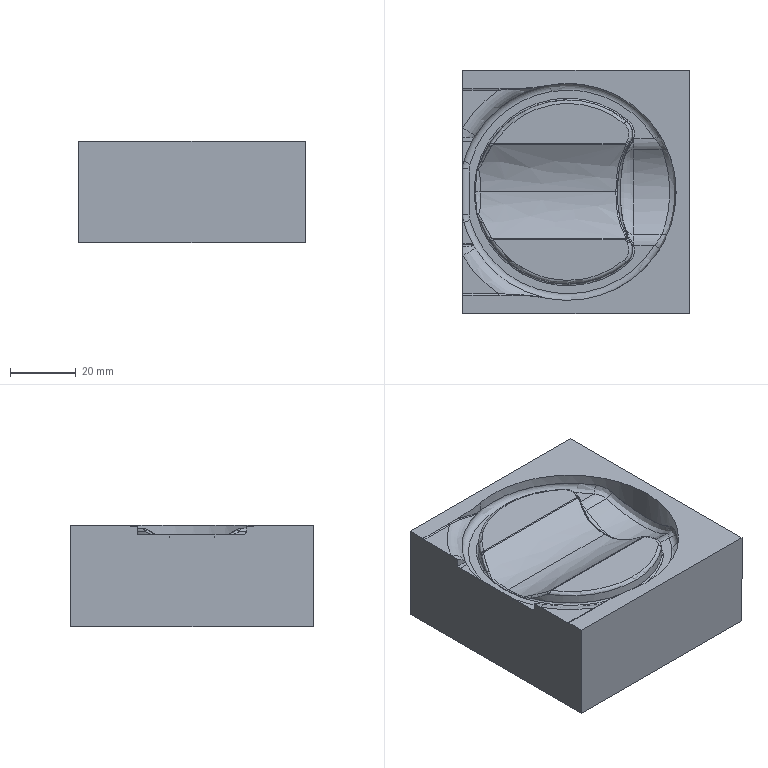NC program | NX | posted with a generic post | part box 69 x 74 x 31.001 mm
Lines 1 to 1116 of 31411:
N10 G17 G21 G94 G90
(CAVITY_MILL , TOOL : D10)
N12 T00 M6
N14 G54
N16 G17 G0 G90 X-5. Y37. S3000 M3
N18 G43 Z10.005 H0
N20 Z0.05
N22 G94 G1 Z-0.15 F2500.
N24 X26.
N26 Y36.067
N28 G2 X31.65 Y35.183 R81.15
N30 G3 X31.65 Y38.817 R-1.85
N32 G2 X26. Y37.933 R81.15
N34 G1 Y37.
N36 X19.5
N38 Y30.081
N40 G2 X30.42 Y28.801 R74.65
N42 G3 X30.42 Y45.199 R-8.35
N44 G2 X19.5 Y43.919 R74.65
N46 G1 Y37.
N48 X13.
N50 Y23.838
N52 G3 X15.404 Y23.65 R100.064
N54 G1 X16.292
N56 G2 X29.19 Y22.418 R68.15
N58 G3 X29.19 Y51.582 R-14.85
N60 G2 X16.292 Y50.35 R68.15
N62 G1 X15.325
N64 X13. Y50.167
N66 Y37.
N68 X6.5
N70 Y17.473
N72 X11.279
N74 X11.596 Y17.442
N76 G3 X15.193 Y17.15 R106.564
N78 G1 X16.292
N80 G2 X27.959 Y16.036 R61.65
N82 G3 X27.959 Y57.964 R-21.35
N84 G2 X16.292 Y56.85 R61.65
N86 G1 X15.069
N88 X10.976 Y56.527
N90 X6.5
N92 Y37.
N94 X0.
N96 Y10.973
N98 X10.961
N100 G3 X14.988 Y10.65 R113.064
N102 G1 X16.292
N104 G2 X26.729 Y9.653 R55.15
N106 G3 X26.729 Y64.347 R-27.85
N108 G2 X16.292 Y63.35 R55.15
N110 G1 X14.813
N112 X10.72 Y63.027
N114 X0.
N116 Y37.
N118 X-5.
N120 Z0.05
N122 G0 Z0.305
N124 Z-0.2
N126 G1 Z-0.4
N128 X33.85
N130 G3 X31.65 Y38.817 R1.85
N132 G2 X27.22 Y38.089 R81.15
N134 X26.569 Y37.006 R31.307
N136 X27.225 Y35.91 R31.167
N138 X31.65 Y35.183 R81.15
N140 G3 X33.85 Y37. R1.85
N142 G1 X40.35
N144 G3 X30.42 Y45.199 R8.35
N146 G2 X23.219 Y44.172 R74.65
N148 G3 X22.617 Y43.364 R11.338
N150 G1 X22.107 Y42.289
N152 G2 X19.5 Y38.251 R24.807
N154 G1 Y35.767
N156 G2 X22.41 Y31.101 R24.667
N158 G1 X22.67 Y30.558
N160 G3 X23.219 Y29.828 R11.338
N162 G2 X30.42 Y28.801 R74.65
N164 G3 X40.35 Y37. R8.35
N166 G1 X46.85
N168 G3 X29.19 Y51.582 R14.85
N170 G2 X20.304 Y50.468 R68.15
N172 G3 X16.935 Y46.55 R17.838
N174 G1 X16.288 Y45.188
N176 G2 X13. Y40.71 R18.307
N178 G1 Y33.31
N180 G2 X16.546 Y28.296 R18.167
N182 G1 X17.004 Y27.341
N184 G3 X20.304 Y23.532 R17.838
N186 G2 X29.19 Y22.418 R68.15
N188 G3 X46.85 Y37. R14.85
N190 G1 X53.35
N192 G3 X27.959 Y57.964 R21.35
N194 G2 X17.949 Y56.872 R61.65
N196 G3 X11.22 Y49.668 R24.338
N198 G1 X10.48 Y48.111
N200 G2 X6.5 Y43.763 R11.807
N202 G1 Y30.253
N204 G2 X10.682 Y25.492 R11.667
N206 G1 X11.303 Y24.195
N208 G3 X17.949 Y17.128 R24.338
N210 G2 X27.959 Y16.036 R61.65
N212 G3 X53.35 Y37. R21.35
N214 G1 X59.85
N216 G3 X26.729 Y64.347 R27.85
N218 G2 X16.292 Y63.35 R55.15
N220 G1 X16.095
N222 X15.926 Y63.318
N224 G3 X5.66 Y53.037 R30.838
N226 G1 X5.468 Y52.708
N228 X4.696 Y51.083
N230 G2 X0. Y48.349 R5.307
N232 G1 Y25.651
N234 G2 X0.837 Y25.584 R5.161
N236 X4.818 Y22.689 R5.167
N238 G1 X5.558 Y21.142
N240 X5.66 Y20.963
N242 G3 X15.979 Y10.65 R30.838
N244 G1 X16.292
N246 G2 X26.729 Y9.653 R55.15
N248 G3 X59.85 Y37. R27.85
N250 G1 X54.85
N252 Z-0.2
N254 G0 Z0.15
N256 X-5.
N258 Z-0.45
N260 G1 Z-0.65
N262 X33.85
N264 G3 X31.65 Y38.817 R1.85
N266 G2 X27.925 Y38.188 R81.15
N268 X27.213 Y36.999 R31.319
N270 X27.924 Y35.812 R31.317
N272 X31.65 Y35.183 R81.15
N274 G3 X33.85 Y37. R1.85
N276 G1 X40.35
N278 G3 X30.42 Y45.199 R8.35
N280 G2 X24.124 Y44.262 R74.65
N282 G3 X23.065 Y42.91 R10.713
N284 G2 X19.5 Y37.467 R24.819
N286 G1 Y36.532
N288 G2 X23.061 Y31.095 R24.817
N290 G3 X24.124 Y29.738 R10.713
N292 G2 X30.42 Y28.801 R74.65
N294 G3 X40.35 Y37. R8.35
N296 G1 X46.85
N298 G3 X29.19 Y51.582 R14.85
N300 G2 X21.372 Y50.54 R68.15
N302 G3 X17.359 Y46.052 R17.213
N304 G2 X13. Y40.094 R18.319
N306 G1 Y33.905
N308 G2 X17.355 Y27.955 R18.317
N310 G3 X21.372 Y23.46 R17.213
N312 G2 X29.19 Y22.418 R68.15
N314 G3 X46.85 Y37. R14.85
N316 G1 X53.35
N318 G3 X27.959 Y57.964 R21.35
N320 G2 X19.128 Y56.915 R61.65
N322 G3 X11.746 Y49.332 R23.713
N324 X11.483 Y48.832 R4.509
N326 G2 X6.5 Y43.371 R11.819
N328 G1 Y30.628
N330 G2 X11.477 Y25.178 R11.817
N332 G3 X11.746 Y24.668 R4.637
N334 X19.128 Y17.085 R23.713
N336 G2 X27.959 Y16.036 R61.65
N338 G3 X53.35 Y37. R21.35
N340 G1 X59.85
N342 G3 X26.729 Y64.347 R27.85
N344 G2 X17.233 Y63.358 R55.15
N346 G3 X6.194 Y52.712 R30.213
N348 X5.552 Y51.492 R11.009
N350 G2 X0.663 Y48.35 R5.319
N352 G1 X0.
N354 Y25.65
N356 X0.666
N358 G2 X5.549 Y22.513 R5.317
N360 G3 X6.194 Y21.288 R11.137
N362 X17.233 Y10.642 R30.213
N364 G2 X26.729 Y9.653 R55.15
N366 G3 X59.85 Y37. R27.85
N368 G1 X54.85
N370 Z-0.45
N372 G0 Z-0.1
N374 X-5.
N376 Z-0.7
N378 G1 Z-0.9
N380 X33.85
N382 G3 X31.65 Y38.817 R1.85
N384 G2 X28.439 Y38.264 R81.15
N386 X27.686 Y37. R31.284
N388 X28.438 Y35.736 R31.257
N390 X31.65 Y35.183 R81.15
N392 G3 X33.85 Y37. R1.85
N394 G1 X40.35
N396 G3 X30.42 Y45.199 R8.35
N398 G2 X24.823 Y44.339 R74.65
N400 G3 X23.424 Y42.641 R10.265
N402 G1 X22.973 Y41.811
N404 G2 X19.565 Y37.001 R24.784
N406 X22.955 Y32.22 R24.757
N408 G1 X23.421 Y31.364
N410 G3 X24.823 Y29.661 R10.265
N412 G2 X30.42 Y28.801 R74.65
N414 G3 X40.35 Y37. R8.35
N416 G1 X46.85
N418 G3 X29.19 Y51.582 R14.85
N420 G2 X22.206 Y50.607 R68.15
N422 G3 X17.826 Y45.954 R16.765
N424 G1 X17.261 Y44.912
N426 G2 X13. Y39.675 R18.284
N428 G1 Y34.329
N430 G2 X17.245 Y29.115 R18.257
N432 G1 X17.824 Y28.05
N434 G3 X22.206 Y23.393 R16.765
N436 G2 X29.19 Y22.418 R68.15
N438 G3 X46.85 Y37. R14.85
N440 G1 X53.35
N442 G3 X27.959 Y57.964 R21.35
N444 G2 X20.056 Y56.965 R61.65
N446 G3 X12.207 Y49.228 R23.265
N448 G1 X11.548 Y48.013
N450 G2 X6.5 Y43.114 R11.784
N452 G1 Y30.89
N454 G2 X11.534 Y26.01 R11.757
N456 G1 X12.206 Y24.774
N458 G3 X20.056 Y17.035 R23.265
N460 G2 X27.959 Y16.036 R61.65
N462 G3 X53.35 Y37. R21.35
N464 G1 X59.85
N466 G3 X26.729 Y64.347 R27.85
N468 G2 X18.221 Y63.384 R55.15
N470 G3 X6.576 Y52.479 R29.765
N472 G1 X5.835 Y51.113
N474 G2 X1.191 Y48.35 R5.284
N476 G1 X0.
N478 Y25.65
N480 X1.206
N482 G2 X5.824 Y22.904 R5.257
N484 G1 X6.576 Y21.521
N486 G3 X18.221 Y10.616 R29.765
N488 G2 X26.729 Y9.653 R55.15
N490 G3 X59.85 Y37. R27.85
N492 G1 X54.85
N494 Z-0.7
N496 G0 Z-0.35
N498 X-5. Y36.999
N500 Z-0.95
N502 G1 Z-1.15
N504 X6.5
N506 Y34.278
N508 G2 X8.893 Y34.52 R11.975
N510 G1 X49.414 Y34.521
N512 G2 X53.136 Y33.986 R12.122
N514 G3 X53.136 Y40.015 R21.35
N516 G2 X49.411 Y39.48 R12.106
N518 G1 X9.291
N520 X8.714 Y39.486
N522 G2 X6.5 Y39.719 R11.904
N524 G1 Y36.999
N526 X0.
N528 Y25.65
N530 X1.623
N532 G2 X4.035 Y25.069 R5.49
N534 X8.893 Y28.02 R5.475
N536 G1 X49.464 Y28.021
N538 G2 X54.095 Y25.737 R5.622
N540 G1 X54.555 Y25.01
N542 G2 X55.793 Y22.525 R11.904
N544 G3 X55.773 Y51.507 R27.85
N546 G2 X54.057 Y48.217 R12.539
N548 X49.464 Y45.98 R5.606
N550 G1 X9.327
N552 X8.786 Y45.986
N554 G2 X4.036 Y48.927 R5.404
N556 X1.617 Y48.35 R5.62
N558 G1 X0.
N560 Y36.999
N562 X-5.
N564 Z-0.95
N566 G0 Z-0.6
N568 Y37.001
N570 Z-1.2
N572 G1 Z-1.4
N574 X6.5
N576 Y34.758
N578 G2 X8.565 Y34.932 R11.933
N580 G1 X49.398 Y34.935
N582 G2 X53.184 Y34.344 R12.425
N584 G3 X53.184 Y39.655 R21.35
N586 G2 X49.401 Y39.065 R12.417
N588 G1 X8.561 Y39.068
N590 G2 X6.5 Y39.244 R11.951
N592 G1 Y37.001
N594 X0.
N596 Y25.65
N598 X1.979
N600 G2 X3.65 Y25.378 R5.705
N602 X8.555 Y28.432 R5.433
N604 G1 X49.399 Y28.435
N606 G2 X54.258 Y25.9 R5.925
N608 X55.949 Y22.784 R15.835
N610 G3 X55.952 Y51.21 R27.85
N612 G2 X54.285 Y48.139 R17.009
N614 X49.402 Y45.565 R5.917
N616 G1 X8.555 Y45.568
N618 G2 X3.649 Y48.619 R5.451
N620 X1.98 Y48.35 R6.113
N622 G1 X0.
N624 Y37.001
N626 X-5.
N628 Z-1.2
N630 G0 Z-0.85
N632 Y37. Z-1.45
N634 G1 Z-1.65
N636 X6.5
N638 Y35.216
N640 G2 X8.26 Y35.347 R11.898
N642 G1 X49.127
N644 G2 X53.222 Y34.666 R12.652
N646 G3 X53.222 Y39.335 R21.35
N648 G2 X49.116 Y38.653 R12.684
N650 G1 X8.259
N652 G2 X6.5 Y38.784 R11.896
N654 G1 Y37.
N656 X0.
N658 Y25.65
N660 X2.289
N662 X2.381 Y25.648
N664 X3.152 Y25.576
N666 X3.288 Y25.551
N668 G2 X8.26 Y28.847 R5.398
N670 G1 X49.127
N672 G2 X54.074 Y26.352 R6.152
N674 X56.034 Y22.928 R16.956
N676 G3 X56.027 Y51.083 R27.85
N678 G2 X54.111 Y47.69 R16.733
N680 X49.116 Y45.153 R6.184
N682 G1 X8.259
N684 G2 X3.289 Y48.448 R5.396
N686 X2.29 Y48.35 R5.432
N688 G1 X0.
N690 Y37.
N692 X-5.
N694 Z-1.45
N696 G0 Z-1.1
N698 Y37.001 Z-1.7
N700 G1 Z-1.9
N702 X6.5
N704 Y35.661
N706 G2 X8.034 Y35.759 R11.939
N708 G1 X48.917
N710 G2 X53.255 Y34.993 R12.654
N712 G3 X53.255 Y39.008 R21.35
N714 G2 X48.915 Y38.241 R12.654
N716 G1 X8.001 Y38.246
N718 G2 X6.5 Y38.341 R11.866
N720 G1 Y37.001
N722 X0.
N724 Y25.65
N726 X0.065
N728 X2.562
N730 X2.908 Y25.64
N732 G2 X8.034 Y29.259 R5.439
N734 G1 X48.917
N736 G2 X53.798 Y26.853 R6.154
N738 X56.067 Y22.986 R18.085
N740 G3 X56.066 Y51.015 R27.85
N742 G2 X53.81 Y47.162 R18.369
N744 X48.916 Y44.741 R6.154
N746 G1 X8.001 Y44.746
N748 G2 X2.932 Y48.353 R5.366
N750 G1 X2.562 Y48.35
N752 X0.
N754 Y37.001
N756 X-5.
N758 Z-1.7
N760 G0 Z-1.35
N762 Y36.999
N764 Z-1.95
N766 G1 Z-2.15
N768 X6.5
N770 Y36.099
N772 G2 X7.749 Y36.171 R11.965
N774 G1 X48.669 Y36.172
N776 G2 X53.284 Y35.323 R12.569
N778 G3 X53.284 Y38.676 R21.35
N780 G2 X48.668 Y37.828 R12.565
N782 G1 X7.781
N784 G2 X6.5 Y37.898 R11.903
N786 G1 Y36.999
N788 X0.
N790 Y25.706
N792 G2 X2.559 Y25.711 R40.064
N794 X7.784 Y29.672 R5.465
N796 G1 X48.692
N798 G2 X53.534 Y27.33 R6.069
N800 X56.082 Y23.011 R21.841
N802 G3 X56.078 Y50.996 R27.85
N804 G2 X53.534 Y46.67 R21.181
N806 X48.692 Y44.328 R6.065
N808 G1 X7.784
N810 G2 X2.564 Y48.35 R5.403
N812 G1 X0.
N814 Y36.999
N816 X-5.
N818 Z-1.95
N820 G0 Z-1.6
N822 Y37. Z-2.2
N824 G1 Z-2.4
N826 X6.5
N828 Y36.534
N830 G2 X7.591 Y36.583 R11.963
N832 G1 X48.779 Y36.582
N834 G2 X53.308 Y35.657 R12.355
N836 G3 X53.307 Y38.352 R21.35
N838 G2 X48.551 Y37.417 R12.557
N840 G1 X7.593 Y37.416
N842 G2 X6.5 Y37.466 R11.965
N844 G1 Y37.
N846 X0.
N848 Y25.824
N850 X0.065 Y25.823
N852 X1.978 Y25.826
N854 X2.261 Y25.82
N856 G2 X7.591 Y30.083 R5.463
N858 G1 X48.692
N860 G2 X52.593 Y28.523 R5.855
N862 X53.717 Y27.222 R7.773
N864 X56.092 Y23.028 R27.85
N866 G3 X56.088 Y50.979 R27.85
N868 G2 X53.46 Y46.426 R25.701
N870 X48.551 Y43.917 R6.057
N872 G1 X7.593 Y43.916
N874 G2 X2.226 Y48.35 R5.465
N876 G1 X0.
N878 Y37.
N880 X-5.
N882 Z-2.2
N884 G0 Z-1.85
N886 Z-2.45
N888 G1 Z-2.65
N890 X6.5
N892 Y36.966
N894 G2 X7.36 Y36.997 R11.955
N896 G1 X48.376 Y36.998
N898 G2 X53.326 Y35.98 R12.535
N900 G3 X53.326 Y38.019 R21.35
N902 G2 X48.388 Y37.002 R12.498
N904 G1 X7.375
N906 G2 X6.5 Y37.034 R11.983
N908 G1 Y37.
N910 X0.
N912 Y25.979
N914 X0.065
N916 X1.987 Y25.983
N918 G2 X7.361 Y30.497 R5.455
N920 G1 X48.376 Y30.498
N922 G2 X53.311 Y27.938 R6.035
N924 X55.09 Y25.01 R25.431
N926 X56.102 Y23.045 R17.528
N928 G3 X56.098 Y50.961 R27.85
N930 G2 X55.09 Y48.99 R14.938
N932 X53.253 Y45.991 R23.408
N934 X48.388 Y43.502 R5.998
N936 G1 X7.375
N938 G2 X1.929 Y48.35 R5.483
N940 G1 X0.
N942 Y37.
N944 X-5.
N946 Z-2.45
N948 G0 Z-2.1
N950 Y37.004
N952 Z-2.7
N954 G1 Z-2.9
N956 X51.388
N958 G2 X53.339 Y36.314 R12.466
N960 G3 X53.339 Y37.699 R21.35
N962 G2 X51.388 Y37.004 R12.627
N964 G1 X46.51 Y35.908
N966 X7.011 Y35.901
N968 X6.91 Y35.9
N970 G3 X5. Y35.684 R10.431
N972 G1 Y38.315
N974 G3 X6.882 Y38.095 R10.482
N976 G1 X7.011 Y38.093
N978 X46.508 Y38.091
N980 G3 X46.51 Y35.908 R5.
N982 G1 X51.388 Y37.004
N984 X49.735 Y30.718
N986 G2 X52.551 Y29.048 R5.966
N988 X53.884 Y27.218 R11.566
N990 X56.111 Y23.062 R59.347
N992 G3 X56.107 Y50.945 R27.85
N994 G2 X54.867 Y48.543 R26.342
N996 X52.937 Y45.397 R20.8
N998 X48.692 Y43.104 R6.127
N1000 G1 X47.92 Y43.091
N1002 X7.012 Y43.093
N1004 G2 X1.677 Y48.35 R5.482
N1006 G1 X0.
N1008 Y26.226
N1010 X1.749 Y26.264
N1012 G2 X7.012 Y30.901 R5.431
N1014 G1 X47.92 Y30.908
N1016 X48.692 Y30.896
N1018 G2 X49.735 Y30.718 R5.966
N1020 G1 X51.007 Y35.554
N1022 Z-2.7
N1024 G0 Z-2.35
N1026 X51.836 Y30.549
N1028 Z-2.7
N1030 G3 X52.977 Y37.154 Z-3.15 R-4.
N1032 G2 X52.601 Y37. R12.461
N1034 G1 X47.643 Y36.357
N1036 X10.156 Y36.354
N1038 Y37.639
N1040 X47.643 Y37.642
N1042 G3 X47.643 Y36.357 R5.
N1044 G1 X52.601 Y37.
N1046 G2 X53.348 Y36.679 R12.457
N1048 G3 X53.348 Y37.321 R21.35
N1050 G2 X52.977 Y37.154 R12.461
N1052 G1 X50.409 Y43.126
N1054 G2 X47.92 Y42.642 R5.961
N1056 G1 X7.012 Y42.639
N1058 X5.468 Y42.832
N1060 X5.156 Y42.926
N1062 Y31.075
N1064 X5.468 Y31.167
N1066 X7.012 Y31.354
N1068 X47.92 Y31.357
N1070 G2 X52.937 Y28.818 R5.957
N1072 X54.867 Y25.486 R27.456
N1074 X56.109 Y23.088 R28.096
N1076 G1 X56.467 Y23.697
N1078 G3 X56.394 Y50.437 R27.85
N1080 G1 X56.373 Y50.465
N1082 X56.111 Y50.92
N1084 G2 X54.867 Y48.513 R27.797
N1086 X52.937 Y45.183 R28.593
N1088 X50.409 Y43.126 R5.961
N1090 G1 X52.384 Y38.532
N1092 Z-2.95
N1094 G0 Z-2.6
N1096 X27.197 Y41.34
N1098 Z-2.95
N1100 G3 X32.815 Y37.682 Z-3.4 R-4.
N1102 G1 X28.815
N1104 X9.693 Y37.681
N1106 Y36.315
N1108 X47.934 Y36.318
N1110 G2 X55.079 Y33.451 R10.467
N1112 G3 X55.079 Y40.55 R23.35
N1114 G2 X47.937 Y37.682 R10.478
N1116 G1 X28.815
N1118 X28.814 Y42.182
N1120 X7.012 Y42.181
N1122 X5.314 Y42.353
N1124 X5.193 Y42.383
N1126 Y31.602
N1128 X5.468 Y31.681
N1130 X7.012 Y31.815
N1132 X47.92 Y31.818
N1134 G2 X52.937 Y29.021 R5.967
N1136 X54.867 Y25.515 R34.654
N1138 X56.1 Y23.145 R30.773
N1140 G3 X57.012 Y24.751 R30.013
N1142 X57.022 Y49.227 R27.85
N1144 X56.106 Y50.866 R47.983
N1146 G2 X54.867 Y48.485 R30.945
N1148 X53.025 Y45.123 R37.413
N1150 X47.92 Y42.182 R5.978
N1152 G1 X28.814
N1154 X28.815 Y37.182
N1156 Z-3.2
N1158 G0 Z-2.85
N1160 X30.525 Y33.152
N1162 Z-3.2
N1164 G3 X24.909 Y36.812 Z-3.65 R-4.
N1166 G1 X28.909 Y36.811
N1168 X47.184 Y36.807
N1170 X48.053 Y36.793
N1172 G2 X55.119 Y33.72 R10.583
N1174 G3 X55.118 Y40.282 R23.35
N1176 G2 X48.038 Y37.194 R10.637
N1178 G1 X47.155 Y37.191
N1180 X9.765 Y37.192
N1182 Y36.81
N1184 X13.184 Y36.815
N1186 X28.909 Y36.811
N1188 X28.908 Y32.311
N1190 X47.148 Y32.307
N1192 X47.92 Y32.295
N1194 G2 X52.937 Y29.235 R6.083
N1196 X54.867 Y25.544 R49.441
N1198 X56.082 Y23.225 R35.757
N1200 G3 X57.173 Y25.085 R44.873
N1202 X57.162 Y48.937 R27.85
N1204 X56.083 Y50.775 R50.152
N1206 G2 X54.867 Y48.456 R34.738
N1208 X52.937 Y44.764 R53.51
N1210 X47.92 Y41.693 R6.137
N1212 G1 X47.148 Y41.691
N1214 X7.012 Y41.692
N1216 X5.265 Y41.831
N1218 Y32.159
N1220 X7.012 Y32.306
N1222 X13.186 Y32.315
N1224 X28.908 Y32.311
N1226 X28.909 Y37.311
N1228 Z-3.45
N1230 G0 Z-3.1
N1232 X49.732 Y40.661
N1234 Z-3.45
N1236 G3 X55.35 Y37.003 Z-3.9 R-4.
N1238 X55.16 Y39.969 R23.35
N1240 G2 X50.109 Y37. R10.428
N1242 X55.161 Y34.037 R10.42
N1244 G3 X55.35 Y37.003 R23.35
N1246 G1 X59.85 Y37.004
N1248 G3 X57.474 Y48.255 R27.85
N1250 X56.305 Y50.232 R15.565
N1252 G1 X56.283 Y50.257
N1254 X56.041 Y50.643
N1256 G2 X54.867 Y48.428 R41.768
N1258 X52.808 Y44.349 R56.972
N1260 X48.474 Y41.255 R5.928
N1262 G1 X47.92 Y41.185
N1264 X6.24 Y41.181
N1266 X5.377 Y41.259
N1268 Y32.771
N1270 X5.37 Y32.758
N1272 X5.379 Y32.746
N1274 X5.394 Y32.751
N1276 X6.24 Y32.817
N1278 X47.578 Y32.812
N1280 G2 X52.757 Y29.758 R5.92
N1282 X54.867 Y25.573 R61.015
N1284 X56.041 Y23.356 R46.33
N1286 G3 X57.483 Y25.765 R20.559
N1288 X59.85 Y37.004 R27.85
N1290 G1 X54.85 Y37.003
N1292 Z-3.7
N1294 G0 Z-3.35
N1296 X49.733 Y40.659
N1298 Z-3.7
N1300 G3 X55.35 Y37. Z-4.15 R-4.
N1302 X55.199 Y39.647 R23.35
N1304 G2 X51.581 Y37. R10.405
N1306 X55.2 Y34.353 R10.407
N1308 G3 X55.35 Y37. R23.35
N1310 G1 X59.85
N1312 G3 X57.604 Y47.956 R27.85
N1314 X56.884 Y49.171 R8.091
N1316 G1 X55.991 Y50.413
N1318 X55.98 Y50.464
N1320 G2 X54.777 Y48.217 R247.416
N1322 X52.576 Y43.698 R55.038
N1324 X47.391 Y40.619 R5.905
N1326 G1 X6.24 Y40.623
N1328 X5.538 Y40.648
N1330 Y33.356
N1332 X6.24 Y33.378
N1334 X47.39 Y33.381
N1336 G2 X52.58 Y30.296 R5.907
N1338 X54.777 Y25.783 R55.784
N1340 X55.969 Y23.539 R128.324
N1342 G1 X57.182 Y25.269
N1344 X57.518 Y25.86
N1346 X57.571 Y25.966
N1348 G3 X59.85 Y37. R27.85
N1350 G1 X54.85
N1352 Z-3.95
N1354 G0 Z-3.6
N1356 X50.003 Y40.688
N1358 Z-3.95
N1360 G3 X55.35 Y36.992 Z-4.4 R-3.95
N1362 X55.238 Y39.283 R23.35
N1364 G2 X52.559 Y36.994 R10.472
N1366 X55.236 Y34.7 R10.643
N1368 G3 X55.35 Y36.992 R23.35
N1370 G1 X59.85 Y36.99
N1372 G3 X57.697 Y47.738 R27.85
N1374 X57.269 Y48.429 R3.855
N1376 G1 X55.878 Y50.22
N1378 X54.792 Y48.217
N1380 G2 X52.644 Y43.575 R82.913
N1382 G1 X52.551 Y43.35
N1384 G2 X47.148 Y40.014 R5.972
N1386 G1 X13.958 Y40.004
N1388 X5.765 Y40.02
N1390 Y33.977
N1392 X6.24 Y33.987
N1394 X47.148 Y33.986
N1396 X47.92 Y33.96
N1398 G2 X52.551 Y30.649 R6.143
N1400 X54.791 Y25.783 R108.189
N1402 G1 X54.867 Y25.632
N1404 X55.877 Y23.781
N1406 X57.208 Y25.491
N1408 G3 X57.687 Y26.239 R4.82
N1410 X59.85 Y36.99 R27.85
N1412 G1 X54.85 Y36.992
N1414 Z-4.2
N1416 G0 Z-3.85
N1418 X52.256 Y40.511
N1420 Z-4.2
N1422 G3 X55.35 Y36.988 Z-4.65 R-3.55
N1424 X55.272 Y38.904 R23.35
N1426 G2 X53.389 Y36.987 R11.458
N1428 X54.75 Y35.704 R10.17
N1430 X55.27 Y35.073 R12.165
N1432 G3 X55.35 Y36.988 R23.35
N1434 G1 X59.85 Y36.986
N1436 G3 X57.788 Y47.516 R27.85
N1438 X57.527 Y47.878 R2.271
N1440 G1 X55.736 Y49.906
N1442 G3 X54.284 Y47.032 R19.65
N1444 G2 X52.772 Y43.575 R70.453
N1446 G1 X52.65 Y43.278
N1448 G2 X50.236 Y40.243 R6.958
N1450 X47.148 Y39.354 R5.916
N1452 G1 X7.012 Y39.352
N1454 X6.108 Y39.36
N1456 Y34.638
N1458 X10.871 Y34.662
N1460 X47.126 Y34.646
N1462 G2 X51.376 Y32.727 R5.67
N1464 X52.595 Y30.851 R7.665
N1466 X54.456 Y26.557 R110.926
N1468 G3 X55.727 Y24.111 R18.908
N1470 G1 X57.291 Y25.828
N1472 G3 X57.801 Y26.515 R4.274
N1474 X59.85 Y36.986 R27.85
N1476 G1 X54.85 Y36.989
N1478 Z-4.45
N1480 G0 Z-4.1
N1482 X59.009 Y38.615
N1484 Z-4.45
N1486 G3 X55.35 Y32.998 Z-4.9 R-4.
N1488 G1 Y36.998
N1490 G3 X55.307 Y38.409 R23.35
N1492 G2 X54.087 Y36.996 R10.117
N1494 X55.307 Y35.587 R10.25
N1496 G3 X55.35 Y36.998 R23.35
N1498 G1 X59.85
N1500 G3 X57.884 Y47.278 R27.85
N1502 X55.435 Y49.239 R13.707
N1504 X54.47 Y47.443 R7.765
N1506 G2 X52.577 Y42.802 R243.005
N1508 G1 X52.551 Y42.722
N1510 X52.143 Y41.868
N1512 G2 X47.307 Y38.677 R5.617
N1514 G1 X46.376 Y38.638
N1516 X6.881 Y38.655
N1518 Y35.357
N1520 X46.981 Y35.359
N1522 G2 X52.22 Y31.98 R5.75
N1524 X53.85 Y28.104 R77.922
N1526 G3 X54.933 Y25.547 R37.185
N1528 X55.428 Y24.775 R3.485
N1530 X57.893 Y26.745 R10.686
N1532 X59.85 Y36.998 R27.85
N1534 G1 X54.85
N1536 Z-4.7
N1538 G0 Z-4.35
N1540 X58.978 Y38.682
N1542 Z-4.7
N1544 G3 X55.35 Y32.998 Z-5.148 R-4.
N1546 G1 Y36.998
N1548 G3 X55.336 Y37.818 R23.35
N1550 G2 X54.724 Y36.998 R10.246
N1552 X55.336 Y36.178 R10.25
N1554 G3 X55.35 Y36.998 R23.35
N1556 G1 X59.85
N1558 G3 X58.133 Y46.627 R27.85
N1560 G1 X54.164
N1562 G2 X52.182 Y41.442 R478.886
N1564 X46.826 Y37.78 R5.746
N1566 G1 X9.327 Y37.783
N1568 X9.032 Y37.798
N1570 G3 X9.032 Y36.216 R22.982
N1572 G1 X46.825 Y36.215
N1574 G2 X52.181 Y32.558 R5.75
N1576 X54.164 Y27.373 R387.614
N1578 G1 X58.133
N1580 G3 X59.85 Y36.998 R27.85
N1582 G1 X54.85
N1584 Z-4.948
N1586 G0 Z-4.6
N1588 X58.977 Y38.691
N1590 Z-4.948
N1592 G3 X55.351 Y33.006 Z-5.396 R-4.
N1594 G1 X55.35 Y37.006
N1596 X55.349 Y37.172
N1598 G2 X55.244 Y37.001 R13.61
N1600 G1 X55.349 Y36.839
N1602 X55.35 Y37.006
N1604 X59.85 Y37.007
N1606 G3 X58.354 Y46.004 R27.85
N1608 G1 X53.956
N1610 G3 X52.56 Y42.028 R225.378
N1612 G1 X52.461 Y41.688
N1614 G2 X51.214 Y39.062 R9.11
N1616 X48.17 Y36.999 R5.059
N1618 X52.165 Y33.173 R6.174
N1620 G1 X52.808 Y31.198
N1622 G2 X53.96 Y27.996 R127.362
N1624 G1 X58.354
N1626 G3 X59.85 Y37.007 R27.85
N1628 G1 X54.85 Y37.005
N1630 Z-5.196
N1632 G0 Z-4.848
N1634 X59.334 Y33.708
N1636 Z-5.196
N1638 G3 X52.609 Y33.199 Z-5.644 R-4.
N1640 G1 X56.168 Y28.455
N1642 X58.507
N1644 G3 X58.507 Y45.545 R27.85
N1646 G1 X53.831
N1648 G3 X52.129 Y40.028 R78.489
N1650 G2 X50.359 Y36.999 R6.663
N1652 X52.133 Y33.942 R6.855
N1654 G3 X53.83 Y28.455 R82.211
N1656 G1 X56.168
N1658 Y33.455
N1660 Z-5.444
N1662 G0 Z-5.096
N1664 X56.714 Y33.114
N1666 Z-5.444
N1668 G3 X51.816 Y37.749 Z-5.892 R-4.
N1670 G1 X51.672 Y37.
N1672 X51.671 Y36.992
N1674 G3 X53.738 Y28.825 R67.462
N1676 G1 X58.623
N1678 G3 X58.623 Y45.175 R27.85
N1680 G1 X53.739
N1682 G3 X51.672 Y37. R66.321
N1684 G1 X56.588 Y36.085
N1686 Z-5.692
N1688 G0 Z-5.344
N1690 X58.818 Y33.376
N1692 Z-5.692
N1694 G3 X52.924 Y33.762 Z-6.14 R-3.8
N1696 G1 X56.194 Y29.136
N1698 X58.717
N1700 G3 X58.717 Y44.864 R27.85
N1702 G1 X53.675
N1704 G3 X52.552 Y40.481 R55.129
N1706 X52.552 Y33.519 R16.674
N1708 X53.671 Y29.141 R56.747
N1710 G1 X53.703 Y29.136
N1712 X56.194
N1714 Y34.136
N1716 Z-5.94
N1718 G0 Z-5.592
N1720 X58.617 Y32.904
N1722 Z-5.94
N1724 G3 X53.179 Y33.368 Z-6.388 R-3.7
N1726 G1 X56.211 Y29.432
N1728 X58.802
N1730 G3 X58.802 Y44.568 R27.85
N1732 G1 X53.622
N1734 G3 X52.818 Y41.255 R58.946
N1736 X52.817 Y32.745 R19.658
N1738 X53.62 Y29.432 R62.313
N1740 G1 X56.211
N1742 Y34.432
N1744 Z-6.188
N1746 G0 Z-5.84
N1748 X53.999 Y40.933
N1750 Z-6.188
N1752 G3 X59.159 Y40.112 Z-6.636 R-3.65
N1754 G1 X56.227 Y44.259
N1756 X53.567
N1758 G3 X52.876 Y41.081 R52.068
N1760 X52.875 Y32.931 R22.418
N1762 X53.569 Y29.741 R51.899
N1764 G1 X58.887
N1766 G3 X58.887 Y44.259 R27.85
N1768 G1 X56.227
N1770 Y39.259
N1772 Z-6.436
N1774 G0 Z-6.088
N1776 X54.245 Y40.81
N1778 Z-6.436
N1780 G3 X59.152 Y39.923 Z-6.884 R-3.6
N1782 G1 X56.245 Y43.937
N1784 X53.518
N1786 G3 X52.869 Y40.44 R44.027
N1788 X53.008 Y32.622 R24.38
N1790 X53.519 Y30.063 R72.064
N1792 G1 X58.972
N1794 G3 X58.972 Y43.937 R27.85
N1796 G1 X56.245
N1798 Y38.937
N1800 Z-6.684
N1802 G0 Z-6.336
N1804 X55.936 Y33.502
N1806 Z-6.684
N1808 G3 X52.732 Y37. Z-7.132 R-3.55
N1810 X53.473 Y30.399 R32.689
N1812 G1 X59.056
N1814 G3 X59.056 Y43.601 R27.85
N1816 G1 X53.474
N1818 G3 X52.73 Y37.387 R34.526
N1820 X52.732 Y37. R32.689
N1822 G1 X57.731 Y37.05
N1824 Z-6.932
N1826 G0 Z-6.584
N1828 X54.678 Y40.634
N1830 Z-6.932
N1832 G3 X59.082 Y39.736 Z-7.381 R-3.5
N1834 G1 X56.284 Y43.25
N1836 X53.428
N1838 G3 X53.431 Y30.75 R33.358
N1840 G1 X59.14
N1842 G3 X59.14 Y43.25 R27.85
N1844 G1 X56.284
N1846 Y38.25
N1848 Z-7.181
N1850 G0 Z-6.832
N1852 X56.886 Y31.118
N1854 Z-7.181
N1856 G1 X59.222 Z-7.242
N1858 X59.495 Y32.382 Z-7.276
N1860 X59.837 Y35.454 Z-7.357
N1862 Y38.546 Z-7.437
N1864 X59.495 Y41.618 Z-7.518
N1866 X59.222 Y42.882 Z-7.552
N1868 X56.306 Z-7.629
N1870 X53.391
N1872 G3 X53.392 Y31.118 R35.884
N1874 G1 X59.222
N1876 G3 X59.222 Y42.882 R27.85
N1878 G1 X56.306
N1880 Y37.882
N1882 Z-7.429
N1884 G0 Z-7.081
N1886 X56.237 Y31.505
N1888 Z-7.429
N1890 G1 X59.303 Z-7.509
N1892 X59.558 Y32.773 Z-7.543
N1894 X59.844 Y35.586 Z-7.617
N1896 Y38.414 Z-7.691
N1898 X59.558 Y41.227 Z-7.765
N1900 X59.303 Y42.495 Z-7.799
N1902 X56.327 Z-7.877
N1904 X53.351
N1906 G3 X53.354 Y31.505 R39.736
N1908 G1 X59.303
N1910 G3 X59.303 Y42.495 R27.85
N1912 G1 X56.327
N1914 Y37.495
N1916 Z-7.677
N1918 G0 Z-7.329
N1920 X55.541 Y31.913
N1922 Z-7.677
N1924 G1 X59.382 Z-7.777
N1926 X59.618 Y33.184 Z-7.811
N1928 X59.851 Y35.725 Z-7.878
N1930 Y38.275 Z-7.945
N1932 X59.618 Y40.816 Z-8.011
N1934 X59.382 Y42.087 Z-8.045
N1936 X56.35 Z-8.125
N1938 X53.318
N1940 G3 X53.318 Y31.913 R43.537
N1942 G1 X59.382
N1944 G3 X59.382 Y42.087 R27.85
N1946 G1 X56.35
N1948 Y37.087
N1950 Z-7.925
N1952 G0 Z-7.577
N1954 X59.792 Y35.354
N1956 Z-7.925
N1958 G1 X59.88 Y37. Z-7.968
N1960 X59.721 Y39.977 Z-8.046
N1962 X59.523 Y41.255 Z-8.08
N1964 X59.44 Y41.656 Z-8.091
N1966 X53.333 Z-8.25
N1968 X53.308 Y41.583 Z-8.252
N1970 X53.185 Y40.481 Z-8.281
N1972 X53.06 Y38.816 Z-8.325
N1974 X53.055 Y38.67 Z-8.329
N1976 Y37. Z-8.373
N1978 G3 X53.186 Y33.519 R46.427
N1980 G1 X53.306 Y32.428
N1982 X53.331 Y32.344
N1984 X59.439
N1986 X59.523 Y32.745
N1988 G3 X59.523 Y41.255 R27.85
N1990 G1 X59.44 Y41.656
N1992 X53.333
N1994 X53.308 Y41.583
N1996 X53.185 Y40.481
N1998 G3 X53.055 Y37. R46.427
N2000 G1 X58.055 Y37.001
N2002 Z-8.173
N2004 G0 Z-7.825
N2006 X59.033 Y41.198
N2008 Z-8.173
N2010 G1 X53.434 Z-8.319
N2012 X53.255 Y40.698 Z-8.333
N2014 X53.17 Y40.239 Z-8.346
N2016 X53.16 Y39.708 Z-8.359
N2018 X53.067 Y37.977 Z-8.405
N2020 X53.068 Y36.023 Z-8.456
N2022 X53.162 Y34.293 Z-8.501
N2024 X53.175 Y33.748 Z-8.516
N2026 X53.253 Y33.317 Z-8.527
N2028 X53.43 Y32.802 Z-8.541
N2030 X56.466 Z-8.621
N2032 X59.501
N2034 X59.652 Y33.713
N2036 X59.68 Y33.928
N2038 G3 X59.657 Y40.274 R27.85
N2040 G1 X59.647 Y40.318
N2042 X59.513 Y41.154
N2044 X59.505 Y41.198
N2046 X53.434
N2048 G3 X53.16 Y39.708 R4.688
N2050 X53.162 Y34.293 R50.022
N2052 X53.43 Y32.802 R4.926
N2054 G1 X56.466
N2056 Y37.802
N2058 Z-8.421
N2060 G0 Z-8.073
N2062 X53.495 Y40.585
N2064 Z-8.421
N2066 G1 X53.329 Y40.061 Z-8.435
N2068 X53.243 Y39.612 Z-8.447
N2070 X53.195 Y38.934 Z-8.465
N2072 X53.106 Y37.613 Z-8.5
N2074 Y36.387 Z-8.532
N2076 X53.193 Y35.066 Z-8.566
N2078 X53.243 Y34.383 Z-8.584
N2080 X53.327 Y33.945 Z-8.596
N2082 X53.534 Y33.291 Z-8.614
N2084 X59.545 Z-8.771
N2086 X59.712 Y34.156 Z-8.794
N2088 X59.781 Y35.034 Z-8.818
N2090 X59.85 Y36.012 Z-8.843
N2092 Y36.993 Z-8.869
N2094 G3 X59.781 Y38.955 R27.85
N2096 X59.551 Y40.695 R19.529
N2098 G1 X59.52 Y40.709
N2100 X53.535
N2102 G3 X53.195 Y38.934 R7.679
N2104 X53.193 Y35.066 R29.183
N2106 X53.534 Y33.291 R7.814
N2108 G1 X59.545
N2110 G3 X59.781 Y35.034 R15.764
N2112 X59.85 Y36.993 R27.85
N2114 G1 X54.85 Y36.994
N2116 Z-8.669
N2118 G0 Z10.005
(FACE_MILLING , TOOL : D10)
N2120 X30.644 Y41.635
N2122 Z-0.8
N2124 G1 Z-1.
N2126 Y46.635
N2128 X6.33
N2130 X4.905 Y49.426
N2132 G3 X6.16 Y51.026 R5.4
N2134 G1 X6.482 Y51.651
N2136 X6.895 Y52.38
N2138 G2 X18.447 Y63.136 R29.441
N2140 G1 X18.536 Y63.145
N2142 G3 X26.777 Y64.101 R55.4
N2144 G2 X55.203 Y51.946 R27.6
N2146 G1 X54.5 Y50.362
N2148 X52.266 Y46.635
N2150 X30.644
N2152 Y53.135
N2154 X15.692
N2156 G2 X20.294 Y56.73 R22.941
N2158 G3 X28.007 Y57.719 R61.9
N2160 G2 X45.597 Y53.135 R21.1
N2162 G1 X30.644
N2164 Y41.635
N2166 Z-0.8
N2168 G0 Z10.005
N2170 Y32.365
N2172 Z-0.8
N2174 G1 Z-1.
N2176 Y27.365
N2178 X52.218
N2180 X54.278 Y24.021
N2182 X54.463 Y23.705
N2184 X55.044 Y22.488
N2186 X55.176 Y22.012
N2188 G2 X26.777 Y9.899 R27.6
N2190 G3 X18.487 Y10.857 R55.4
N2192 G1 X18.456 Y10.859
N2194 G2 X6.89 Y21.629 R29.441
N2196 G1 X6.577 Y22.177
N2198 X6.146 Y23.
N2200 G3 X4.904 Y24.575 R5.4
N2202 G1 X6.376 Y27.365
N2204 X30.644
N2206 Y20.865
N2208 X45.597
N2210 G2 X28.007 Y16.281 R21.1
N2212 G3 X20.294 Y17.27 R61.9
N2214 G2 X15.692 Y20.865 R22.941
N2216 G1 X30.644
N2218 Y32.365
N2220 Z-0.8
N2222 G0 Z10.005
N2224 M5